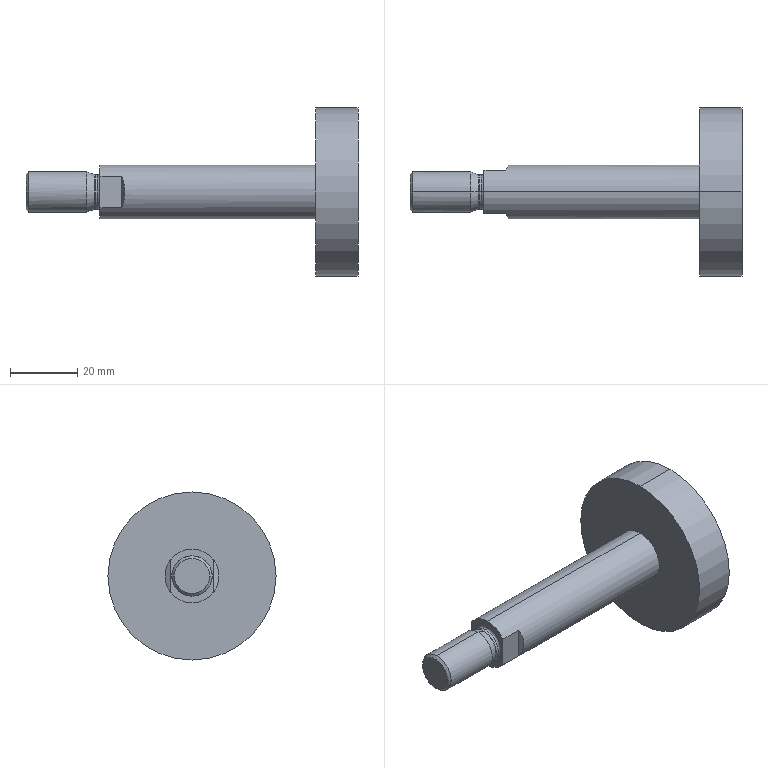Part | SolidWorks | features BaseBody 1 | 1 solid | 24 faces | box 98.8 x 50 x 50 mm | volume 39735 mm3 | cylinder 8 | plane 8 | spline 4 | cone 4 | commonest cylinder face diameters 10.2 x2 12 x2 16 x2 50 x2
STEP:
#1=CARTESIAN_POINT('',(-8.8,0.,5.1));
#2=VERTEX_POINT('',#1);
#3=CARTESIAN_POINT('',(-8.8,0.,-5.1));
#4=VERTEX_POINT('',#3);
#5=CARTESIAN_POINT('',(-8.8,0.,0.));
#6=DIRECTION('',(-1.,0.,0.));
#7=DIRECTION('',(0.,0.,-1.));
#8=AXIS2_PLACEMENT_3D('',#5,#6,#7);
#9=CIRCLE('',#8,5.1);
#10=EDGE_CURVE('',#2,#4,#9,.T.);
#11=ORIENTED_EDGE('',*,*,#10,.F.);
#12=CARTESIAN_POINT('',(-8.2,0.,5.7));
#13=VERTEX_POINT('',#12);
#14=CARTESIAN_POINT('',(-8.8,0.,5.7));
#15=DIRECTION('',(0.,-1.,0.));
#16=DIRECTION('',(0.,0.,1.));
#17=AXIS2_PLACEMENT_3D('',#14,#15,#16);
#18=CIRCLE('',#17,0.6);
#19=EDGE_CURVE('',#2,#13,#18,.T.);
#20=ORIENTED_EDGE('',*,*,#19,.T.);
#21=CARTESIAN_POINT('',(-8.2,0.,-5.7));
#22=VERTEX_POINT('',#21);
#23=CARTESIAN_POINT('',(-8.2,0.,5.7));
#24=CARTESIAN_POINT('',(-8.2,11.4,5.7));
#25=CARTESIAN_POINT('',(-8.2,11.4,-5.7));
#26=CARTESIAN_POINT('',(-8.2,0.,-5.7));
#27=(BOUNDED_CURVE()B_SPLINE_CURVE(3,(#23,#24,#25,#26),.UNSPECIFIED.,.F.,.F.)B_SPLINE_CURVE_WITH_KNOTS((4,4),(0.5,1.),.UNSPECIFIED.)CURVE()GEOMETRIC_REPRESENTATION_ITEM()RATIONAL_B_SPLINE_CURVE((1.,0.3333,0.3333,1.))REPRESENTATION_ITEM(''));
#28=EDGE_CURVE('',#13,#22,#27,.T.);
#29=ORIENTED_EDGE('',*,*,#28,.T.);
#30=CARTESIAN_POINT('',(-8.8,0.,-5.7));
#31=DIRECTION('',(0.,1.,0.));
#32=DIRECTION('',(0.,0.,-1.));
#33=AXIS2_PLACEMENT_3D('',#30,#31,#32);
#34=CIRCLE('',#33,0.6);
#35=EDGE_CURVE('',#4,#22,#34,.T.);
#36=ORIENTED_EDGE('',*,*,#35,.F.);
#37=EDGE_LOOP('',(#11,#20,#29,#36));
#38=FACE_OUTER_BOUND('',#37,.T.);
#39=CARTESIAN_POINT('',(-8.8,0.,-5.1));
#40=CARTESIAN_POINT('',(-8.8,10.2,-5.1));
#41=CARTESIAN_POINT('',(-8.8,10.2,5.1));
#42=CARTESIAN_POINT('',(-8.8,0.,5.1));
#43=CARTESIAN_POINT('',(-8.449,0.,-5.1));
#44=CARTESIAN_POINT('',(-8.449,10.2,-5.1));
#45=CARTESIAN_POINT('',(-8.449,10.2,5.1));
#46=CARTESIAN_POINT('',(-8.449,0.,5.1));
#47=CARTESIAN_POINT('',(-8.2,0.,-5.349));
#48=CARTESIAN_POINT('',(-8.2,10.697,-5.349));
#49=CARTESIAN_POINT('',(-8.2,10.697,5.349));
#50=CARTESIAN_POINT('',(-8.2,0.,5.349));
#51=CARTESIAN_POINT('',(-8.2,0.,-5.7));
#52=CARTESIAN_POINT('',(-8.2,11.4,-5.7));
#53=CARTESIAN_POINT('',(-8.2,11.4,5.7));
#54=CARTESIAN_POINT('',(-8.2,0.,5.7));
#55=(BOUNDED_SURFACE()B_SPLINE_SURFACE(3,3,((#39,#40,#41,#42),(#43,#44,#45,#46),(#47,#48,#49,#50),(#51,#52,#53,#54)),.UNSPECIFIED.,.F.,.F.,.F.)B_SPLINE_SURFACE_WITH_KNOTS((4,4),(4,4),(0.,1.),(0.,1.),.UNSPECIFIED.)GEOMETRIC_REPRESENTATION_ITEM()RATIONAL_B_SPLINE_SURFACE(((1.,0.3333,0.3333,1.),(0.8047,0.2682,0.2682,0.8047),(0.8047,0.2682,0.2682,0.8047),(1.,0.3333,0.3333,1.)))REPRESENTATION_ITEM('')SURFACE());
#56=ADVANCED_FACE('',(#38),#55,.F.);
#57=CARTESIAN_POINT('',(-9.799,0.,5.136));
#58=VERTEX_POINT('',#57);
#59=CARTESIAN_POINT('',(-9.799,0.,-5.136));
#60=VERTEX_POINT('',#59);
#61=CARTESIAN_POINT('',(-9.799,0.,0.));
#62=DIRECTION('',(-1.,0.,0.));
#63=DIRECTION('',(0.,0.,-1.));
#64=AXIS2_PLACEMENT_3D('',#61,#62,#63);
#65=CIRCLE('',#64,5.136);
#66=EDGE_CURVE('',#58,#60,#65,.T.);
#67=ORIENTED_EDGE('',*,*,#66,.F.);
#68=CARTESIAN_POINT('',(-9.594,0.,5.1));
#69=VERTEX_POINT('',#68);
#70=CARTESIAN_POINT('',(-9.594,0.,5.7));
#71=DIRECTION('',(0.,-1.,0.));
#72=DIRECTION('',(0.,0.,1.));
#73=AXIS2_PLACEMENT_3D('',#70,#71,#72);
#74=CIRCLE('',#73,0.6);
#75=EDGE_CURVE('',#58,#69,#74,.T.);
#76=ORIENTED_EDGE('',*,*,#75,.T.);
#77=CARTESIAN_POINT('',(-9.594,0.,-5.1));
#78=VERTEX_POINT('',#77);
#79=CARTESIAN_POINT('',(-9.594,0.,0.));
#80=DIRECTION('',(1.,0.,0.));
#81=DIRECTION('',(0.,0.,1.));
#82=AXIS2_PLACEMENT_3D('',#79,#80,#81);
#83=CIRCLE('',#82,5.1);
#84=EDGE_CURVE('',#78,#69,#83,.T.);
#85=ORIENTED_EDGE('',*,*,#84,.F.);
#86=CARTESIAN_POINT('',(-9.594,0.,-5.7));
#87=DIRECTION('',(0.,1.,0.));
#88=DIRECTION('',(0.,0.,-1.));
#89=AXIS2_PLACEMENT_3D('',#86,#87,#88);
#90=CIRCLE('',#89,0.6);
#91=EDGE_CURVE('',#60,#78,#90,.T.);
#92=ORIENTED_EDGE('',*,*,#91,.F.);
#93=EDGE_LOOP('',(#67,#76,#85,#92));
#94=FACE_OUTER_BOUND('',#93,.T.);
#95=CARTESIAN_POINT('',(-9.799,0.,-5.136));
#96=CARTESIAN_POINT('',(-9.799,10.272,-5.136));
#97=CARTESIAN_POINT('',(-9.799,10.272,5.136));
#98=CARTESIAN_POINT('',(-9.799,0.,5.136));
#99=CARTESIAN_POINT('',(-9.733,0.,-5.112));
#100=CARTESIAN_POINT('',(-9.733,10.224,-5.112));
#101=CARTESIAN_POINT('',(-9.733,10.224,5.112));
#102=CARTESIAN_POINT('',(-9.733,0.,5.112));
#103=CARTESIAN_POINT('',(-9.664,0.,-5.1));
#104=CARTESIAN_POINT('',(-9.664,10.2,-5.1));
#105=CARTESIAN_POINT('',(-9.664,10.2,5.1));
#106=CARTESIAN_POINT('',(-9.664,0.,5.1));
#107=CARTESIAN_POINT('',(-9.594,0.,-5.1));
#108=CARTESIAN_POINT('',(-9.594,10.2,-5.1));
#109=CARTESIAN_POINT('',(-9.594,10.2,5.1));
#110=CARTESIAN_POINT('',(-9.594,0.,5.1));
#111=(BOUNDED_SURFACE()B_SPLINE_SURFACE(3,3,((#95,#96,#97,#98),(#99,#100,#101,#102),(#103,#104,#105,#106),(#107,#108,#109,#110)),.UNSPECIFIED.,.F.,.F.,.T.)B_SPLINE_SURFACE_WITH_KNOTS((4,4),(4,4),(0.,1.),(0.,1.),.UNSPECIFIED.)GEOMETRIC_REPRESENTATION_ITEM()RATIONAL_B_SPLINE_SURFACE(((1.,0.3333,0.3333,1.),(0.9899,0.33,0.33,0.9899),(0.9899,0.33,0.33,0.9899),(1.,0.3333,0.3333,1.)))REPRESENTATION_ITEM('')SURFACE());
#112=ADVANCED_FACE('',(#94),#111,.F.);
#113=CARTESIAN_POINT('',(56.1,0.,8.));
#114=VERTEX_POINT('',#113);
#115=CARTESIAN_POINT('',(56.1,0.,-8.));
#116=VERTEX_POINT('',#115);
#117=CARTESIAN_POINT('',(56.1,0.,0.));
#118=DIRECTION('',(-1.,0.,0.));
#119=DIRECTION('',(0.,0.,1.));
#120=AXIS2_PLACEMENT_3D('',#117,#118,#119);
#121=CIRCLE('',#120,8.);
#122=EDGE_CURVE('',#114,#116,#121,.T.);
#123=ORIENTED_EDGE('',*,*,#122,.T.);
#124=CARTESIAN_POINT('',(-8.2,0.,-8.));
#125=VERTEX_POINT('',#124);
#126=CARTESIAN_POINT('',(68.6,0.,-8.));
#127=DIRECTION('',(-1.,0.,0.));
#128=VECTOR('',#127,1000.);
#129=LINE('',#126,#128);
#130=EDGE_CURVE('',#116,#125,#129,.T.);
#131=ORIENTED_EDGE('',*,*,#130,.T.);
#132=CARTESIAN_POINT('',(-8.2,6.5,-4.664));
#133=VERTEX_POINT('',#132);
#134=CARTESIAN_POINT('',(-8.2,0.,0.));
#135=DIRECTION('',(1.,0.,0.));
#136=DIRECTION('',(0.,0.,1.));
#137=AXIS2_PLACEMENT_3D('',#134,#135,#136);
#138=CIRCLE('',#137,8.);
#139=EDGE_CURVE('',#125,#133,#138,.T.);
#140=ORIENTED_EDGE('',*,*,#139,.T.);
#141=CARTESIAN_POINT('',(-1.7,6.5,-4.664));
#142=VERTEX_POINT('',#141);
#143=CARTESIAN_POINT('',(68.6,6.5,-4.664));
#144=DIRECTION('',(1.,0.,0.));
#145=VECTOR('',#144,1000.);
#146=LINE('',#143,#145);
#147=EDGE_CURVE('',#133,#142,#146,.T.);
#148=ORIENTED_EDGE('',*,*,#147,.T.);
#149=CARTESIAN_POINT('',(-1.7,6.5,4.664));
#150=VERTEX_POINT('',#149);
#151=CARTESIAN_POINT('',(-1.7,6.5,-4.664));
#152=CARTESIAN_POINT('',(-0.5041,8.571,-1.777));
#153=CARTESIAN_POINT('',(-0.5041,8.571,1.777));
#154=CARTESIAN_POINT('',(-1.7,6.5,4.664));
#155=(BOUNDED_CURVE()B_SPLINE_CURVE(3,(#151,#152,#153,#154),.UNSPECIFIED.,.F.,.F.)B_SPLINE_CURVE_WITH_KNOTS((4,4),(2.519,3.764),.UNSPECIFIED.)CURVE()GEOMETRIC_REPRESENTATION_ITEM()RATIONAL_B_SPLINE_CURVE((1.,0.875,0.875,1.))REPRESENTATION_ITEM(''));
#156=EDGE_CURVE('',#142,#150,#155,.T.);
#157=ORIENTED_EDGE('',*,*,#156,.T.);
#158=CARTESIAN_POINT('',(-8.2,6.5,4.664));
#159=VERTEX_POINT('',#158);
#160=CARTESIAN_POINT('',(68.6,6.5,4.664));
#161=DIRECTION('',(-1.,0.,0.));
#162=VECTOR('',#161,1000.);
#163=LINE('',#160,#162);
#164=EDGE_CURVE('',#150,#159,#163,.T.);
#165=ORIENTED_EDGE('',*,*,#164,.T.);
#166=CARTESIAN_POINT('',(-8.2,0.,8.));
#167=VERTEX_POINT('',#166);
#168=CARTESIAN_POINT('',(-8.2,0.,0.));
#169=DIRECTION('',(1.,0.,0.));
#170=DIRECTION('',(0.,0.,1.));
#171=AXIS2_PLACEMENT_3D('',#168,#169,#170);
#172=CIRCLE('',#171,8.);
#173=EDGE_CURVE('',#159,#167,#172,.T.);
#174=ORIENTED_EDGE('',*,*,#173,.T.);
#175=CARTESIAN_POINT('',(68.6,0.,8.));
#176=DIRECTION('',(-1.,0.,0.));
#177=VECTOR('',#176,1000.);
#178=LINE('',#175,#177);
#179=EDGE_CURVE('',#114,#167,#178,.T.);
#180=ORIENTED_EDGE('',*,*,#179,.F.);
#181=EDGE_LOOP('',(#123,#131,#140,#148,#157,#165,#174,#180));
#182=FACE_OUTER_BOUND('',#181,.T.);
#183=CARTESIAN_POINT('',(68.6,0.,0.));
#184=DIRECTION('',(-1.,0.,0.));
#185=DIRECTION('',(0.,0.,1.));
#186=AXIS2_PLACEMENT_3D('',#183,#184,#185);
#187=CYLINDRICAL_SURFACE('',#186,8.);
#188=ADVANCED_FACE('',(#182),#187,.T.);
#189=CARTESIAN_POINT('',(68.6,0.,25.));
#190=VERTEX_POINT('',#189);
#191=CARTESIAN_POINT('',(68.6,0.,-25.));
#192=VERTEX_POINT('',#191);
#193=CARTESIAN_POINT('',(68.6,0.,0.));
#194=DIRECTION('',(-1.,0.,0.));
#195=DIRECTION('',(0.,0.,1.));
#196=AXIS2_PLACEMENT_3D('',#193,#194,#195);
#197=CIRCLE('',#196,25.);
#198=EDGE_CURVE('',#190,#192,#197,.T.);
#199=ORIENTED_EDGE('',*,*,#198,.T.);
#200=CARTESIAN_POINT('',(56.1,0.,-25.));
#201=VERTEX_POINT('',#200);
#202=CARTESIAN_POINT('',(68.6,0.,-25.));
#203=DIRECTION('',(-1.,0.,0.));
#204=VECTOR('',#203,1000.);
#205=LINE('',#202,#204);
#206=EDGE_CURVE('',#192,#201,#205,.T.);
#207=ORIENTED_EDGE('',*,*,#206,.T.);
#208=CARTESIAN_POINT('',(56.1,0.,25.));
#209=VERTEX_POINT('',#208);
#210=CARTESIAN_POINT('',(56.1,0.,0.));
#211=DIRECTION('',(1.,0.,0.));
#212=DIRECTION('',(0.,0.,1.));
#213=AXIS2_PLACEMENT_3D('',#210,#211,#212);
#214=CIRCLE('',#213,25.);
#215=EDGE_CURVE('',#201,#209,#214,.T.);
#216=ORIENTED_EDGE('',*,*,#215,.T.);
#217=CARTESIAN_POINT('',(68.6,0.,25.));
#218=DIRECTION('',(-1.,0.,0.));
#219=VECTOR('',#218,1000.);
#220=LINE('',#217,#219);
#221=EDGE_CURVE('',#190,#209,#220,.T.);
#222=ORIENTED_EDGE('',*,*,#221,.F.);
#223=EDGE_LOOP('',(#199,#207,#216,#222));
#224=FACE_OUTER_BOUND('',#223,.T.);
#225=CARTESIAN_POINT('',(68.6,0.,0.));
#226=DIRECTION('',(-1.,0.,0.));
#227=DIRECTION('',(0.,0.,1.));
#228=AXIS2_PLACEMENT_3D('',#225,#226,#227);
#229=CYLINDRICAL_SURFACE('',#228,25.);
#230=ADVANCED_FACE('',(#224),#229,.T.);
#231=ORIENTED_EDGE('',*,*,#10,.T.);
#232=CARTESIAN_POINT('',(-7.2,0.,-5.1));
#233=DIRECTION('',(-1.,0.,0.));
#234=VECTOR('',#233,1000.);
#235=LINE('',#232,#234);
#236=EDGE_CURVE('',#4,#78,#235,.T.);
#237=ORIENTED_EDGE('',*,*,#236,.T.);
#238=ORIENTED_EDGE('',*,*,#84,.T.);
#239=CARTESIAN_POINT('',(-7.2,0.,5.1));
#240=DIRECTION('',(-1.,0.,0.));
#241=VECTOR('',#240,1000.);
#242=LINE('',#239,#241);
#243=EDGE_CURVE('',#2,#69,#242,.T.);
#244=ORIENTED_EDGE('',*,*,#243,.F.);
#245=EDGE_LOOP('',(#231,#237,#238,#244));
#246=FACE_OUTER_BOUND('',#245,.T.);
#247=CARTESIAN_POINT('',(-7.2,0.,0.));
#248=DIRECTION('',(-1.,0.,0.));
#249=DIRECTION('',(0.,0.,1.));
#250=AXIS2_PLACEMENT_3D('',#247,#248,#249);
#251=CYLINDRICAL_SURFACE('',#250,5.1);
#252=ADVANCED_FACE('',(#246),#251,.T.);
#253=ORIENTED_EDGE('',*,*,#66,.T.);
#254=CARTESIAN_POINT('',(-12.173,0.,-6.));
#255=VERTEX_POINT('',#254);
#256=CARTESIAN_POINT('',(-12.173,0.,-6.));
#257=DIRECTION('',(-0.9397,0.,-0.342));
#258=VECTOR('',#257,1000.);
#259=LINE('',#256,#258);
#260=EDGE_CURVE('',#60,#255,#259,.T.);
#261=ORIENTED_EDGE('',*,*,#260,.T.);
#262=CARTESIAN_POINT('',(-12.173,0.,6.));
#263=VERTEX_POINT('',#262);
#264=CARTESIAN_POINT('',(-12.173,0.,0.));
#265=DIRECTION('',(1.,0.,0.));
#266=DIRECTION('',(0.,0.,1.));
#267=AXIS2_PLACEMENT_3D('',#264,#265,#266);
#268=CIRCLE('',#267,6.);
#269=EDGE_CURVE('',#255,#263,#268,.T.);
#270=ORIENTED_EDGE('',*,*,#269,.T.);
#271=CARTESIAN_POINT('',(-12.173,0.,6.));
#272=DIRECTION('',(-0.9397,0.,0.342));
#273=VECTOR('',#272,1000.);
#274=LINE('',#271,#273);
#275=EDGE_CURVE('',#58,#263,#274,.T.);
#276=ORIENTED_EDGE('',*,*,#275,.F.);
#277=EDGE_LOOP('',(#253,#261,#270,#276));
#278=FACE_OUTER_BOUND('',#277,.T.);
#279=CARTESIAN_POINT('',(-12.173,0.,0.));
#280=DIRECTION('',(-1.,0.,0.));
#281=DIRECTION('',(0.,0.,1.));
#282=AXIS2_PLACEMENT_3D('',#279,#280,#281);
#283=CONICAL_SURFACE('',#282,6.,0.3491);
#284=ADVANCED_FACE('',(#278),#283,.T.);
#285=ORIENTED_EDGE('',*,*,#269,.F.);
#286=CARTESIAN_POINT('',(-29.433,0.,-6.));
#287=VERTEX_POINT('',#286);
#288=CARTESIAN_POINT('',(-7.2,0.,-6.));
#289=DIRECTION('',(-1.,0.,0.));
#290=VECTOR('',#289,1000.);
#291=LINE('',#288,#290);
#292=EDGE_CURVE('',#255,#287,#291,.T.);
#293=ORIENTED_EDGE('',*,*,#292,.T.);
#294=CARTESIAN_POINT('',(-29.433,6.,0.));
#295=VERTEX_POINT('',#294);
#296=CARTESIAN_POINT('',(-29.433,0.,0.));
#297=DIRECTION('',(1.,0.,0.));
#298=DIRECTION('',(0.,0.,1.));
#299=AXIS2_PLACEMENT_3D('',#296,#297,#298);
#300=CIRCLE('',#299,6.);
#301=EDGE_CURVE('',#287,#295,#300,.T.);
#302=ORIENTED_EDGE('',*,*,#301,.T.);
#303=CARTESIAN_POINT('',(-29.433,0.,6.));
#304=VERTEX_POINT('',#303);
#305=CARTESIAN_POINT('',(-29.433,0.,0.));
#306=DIRECTION('',(1.,0.,0.));
#307=DIRECTION('',(0.,0.,1.));
#308=AXIS2_PLACEMENT_3D('',#305,#306,#307);
#309=CIRCLE('',#308,6.);
#310=EDGE_CURVE('',#295,#304,#309,.T.);
#311=ORIENTED_EDGE('',*,*,#310,.T.);
#312=CARTESIAN_POINT('',(-7.2,0.,6.));
#313=DIRECTION('',(-1.,0.,0.));
#314=VECTOR('',#313,1000.);
#315=LINE('',#312,#314);
#316=EDGE_CURVE('',#263,#304,#315,.T.);
#317=ORIENTED_EDGE('',*,*,#316,.F.);
#318=EDGE_LOOP('',(#285,#293,#302,#311,#317));
#319=FACE_OUTER_BOUND('',#318,.T.);
#320=CARTESIAN_POINT('',(-7.2,0.,0.));
#321=DIRECTION('',(-1.,0.,0.));
#322=DIRECTION('',(0.,0.,1.));
#323=AXIS2_PLACEMENT_3D('',#320,#321,#322);
#324=CYLINDRICAL_SURFACE('',#323,6.);
#325=ADVANCED_FACE('',(#319),#324,.T.);
#326=CARTESIAN_POINT('',(-30.2,5.233,0.));
#327=VERTEX_POINT('',#326);
#328=CARTESIAN_POINT('',(-30.2,-5.233,0.));
#329=VERTEX_POINT('',#328);
#330=CARTESIAN_POINT('',(-30.2,0.,0.));
#331=DIRECTION('',(1.,0.,0.));
#332=DIRECTION('',(0.,1.,0.));
#333=AXIS2_PLACEMENT_3D('',#330,#331,#332);
#334=CIRCLE('',#333,5.233);
#335=EDGE_CURVE('',#327,#329,#334,.T.);
#336=ORIENTED_EDGE('',*,*,#335,.T.);
#337=CARTESIAN_POINT('',(-29.433,-6.,0.));
#338=VERTEX_POINT('',#337);
#339=CARTESIAN_POINT('',(-29.433,-6.,0.));
#340=DIRECTION('',(0.7071,-0.7071,0.));
#341=VECTOR('',#340,1000.);
#342=LINE('',#339,#341);
#343=EDGE_CURVE('',#329,#338,#342,.T.);
#344=ORIENTED_EDGE('',*,*,#343,.T.);
#345=CARTESIAN_POINT('',(-29.433,0.,0.));
#346=DIRECTION('',(1.,0.,0.));
#347=DIRECTION('',(0.,0.,1.));
#348=AXIS2_PLACEMENT_3D('',#345,#346,#347);
#349=CIRCLE('',#348,6.);
#350=EDGE_CURVE('',#304,#338,#349,.T.);
#351=ORIENTED_EDGE('',*,*,#350,.F.);
#352=ORIENTED_EDGE('',*,*,#310,.F.);
#353=CARTESIAN_POINT('',(-29.433,6.,0.));
#354=DIRECTION('',(0.7071,0.7071,0.));
#355=VECTOR('',#354,1000.);
#356=LINE('',#353,#355);
#357=EDGE_CURVE('',#327,#295,#356,.T.);
#358=ORIENTED_EDGE('',*,*,#357,.F.);
#359=EDGE_LOOP('',(#336,#344,#351,#352,#358));
#360=FACE_OUTER_BOUND('',#359,.T.);
#361=CARTESIAN_POINT('',(-29.433,0.,0.));
#362=DIRECTION('',(1.,0.,0.));
#363=DIRECTION('',(0.,1.,0.));
#364=AXIS2_PLACEMENT_3D('',#361,#362,#363);
#365=CONICAL_SURFACE('',#364,6.,0.7854);
#366=ADVANCED_FACE('',(#360),#365,.T.);
#367=ORIENTED_EDGE('',*,*,#130,.F.);
#368=CARTESIAN_POINT('',(56.1,0.,0.));
#369=DIRECTION('',(-1.,0.,0.));
#370=DIRECTION('',(0.,0.,1.));
#371=AXIS2_PLACEMENT_3D('',#368,#369,#370);
#372=CIRCLE('',#371,8.);
#373=EDGE_CURVE('',#116,#114,#372,.T.);
#374=ORIENTED_EDGE('',*,*,#373,.T.);
#375=ORIENTED_EDGE('',*,*,#179,.T.);
#376=CARTESIAN_POINT('',(-8.2,-6.5,4.664));
#377=VERTEX_POINT('',#376);
#378=CARTESIAN_POINT('',(-8.2,0.,0.));
#379=DIRECTION('',(1.,0.,0.));
#380=DIRECTION('',(0.,0.,1.));
#381=AXIS2_PLACEMENT_3D('',#378,#379,#380);
#382=CIRCLE('',#381,8.);
#383=EDGE_CURVE('',#167,#377,#382,.T.);
#384=ORIENTED_EDGE('',*,*,#383,.T.);
#385=CARTESIAN_POINT('',(-1.7,-6.5,4.664));
#386=VERTEX_POINT('',#385);
#387=CARTESIAN_POINT('',(68.6,-6.5,4.664));
#388=DIRECTION('',(1.,0.,0.));
#389=VECTOR('',#388,1000.);
#390=LINE('',#387,#389);
#391=EDGE_CURVE('',#377,#386,#390,.T.);
#392=ORIENTED_EDGE('',*,*,#391,.T.);
#393=CARTESIAN_POINT('',(-1.7,-6.5,-4.664));
#394=VERTEX_POINT('',#393);
#395=CARTESIAN_POINT('',(-1.7,-6.5,4.664));
#396=CARTESIAN_POINT('',(-0.5041,-8.571,1.777));
#397=CARTESIAN_POINT('',(-0.5041,-8.571,-1.777));
#398=CARTESIAN_POINT('',(-1.7,-6.5,-4.664));
#399=(BOUNDED_CURVE()B_SPLINE_CURVE(3,(#395,#396,#397,#398),.UNSPECIFIED.,.F.,.F.)B_SPLINE_CURVE_WITH_KNOTS((4,4),(2.519,3.764),.UNSPECIFIED.)CURVE()GEOMETRIC_REPRESENTATION_ITEM()RATIONAL_B_SPLINE_CURVE((1.,0.875,0.875,1.))REPRESENTATION_ITEM(''));
#400=EDGE_CURVE('',#386,#394,#399,.T.);
#401=ORIENTED_EDGE('',*,*,#400,.T.);
#402=CARTESIAN_POINT('',(-8.2,-6.5,-4.664));
#403=VERTEX_POINT('',#402);
#404=CARTESIAN_POINT('',(68.6,-6.5,-4.664));
#405=DIRECTION('',(-1.,0.,0.));
#406=VECTOR('',#405,1000.);
#407=LINE('',#404,#406);
#408=EDGE_CURVE('',#394,#403,#407,.T.);
#409=ORIENTED_EDGE('',*,*,#408,.T.);
#410=CARTESIAN_POINT('',(-8.2,0.,0.));
#411=DIRECTION('',(1.,0.,0.));
#412=DIRECTION('',(0.,0.,1.));
#413=AXIS2_PLACEMENT_3D('',#410,#411,#412);
#414=CIRCLE('',#413,8.);
#415=EDGE_CURVE('',#403,#125,#414,.T.);
#416=ORIENTED_EDGE('',*,*,#415,.T.);
#417=EDGE_LOOP('',(#367,#374,#375,#384,#392,#401,#409,#416));
#418=FACE_OUTER_BOUND('',#417,.T.);
#419=CARTESIAN_POINT('',(68.6,0.,0.));
#420=DIRECTION('',(-1.,0.,0.));
#421=DIRECTION('',(0.,0.,1.));
#422=AXIS2_PLACEMENT_3D('',#419,#420,#421);
#423=CYLINDRICAL_SURFACE('',#422,8.);
#424=ADVANCED_FACE('',(#418),#423,.T.);
#425=ORIENTED_EDGE('',*,*,#400,.F.);
#426=CARTESIAN_POINT('',(-1.7,-6.5,16.));
#427=DIRECTION('',(0.,0.,-1.));
#428=VECTOR('',#427,1000.);
#429=LINE('',#426,#428);
#430=EDGE_CURVE('',#386,#394,#429,.T.);
#431=ORIENTED_EDGE('',*,*,#430,.T.);
#432=EDGE_LOOP('',(#425,#431));
#433=FACE_OUTER_BOUND('',#432,.T.);
#434=CARTESIAN_POINT('',(5.806,-19.5,16.));
#435=DIRECTION('',(-0.866,-0.5,0.));
#436=DIRECTION('',(0.5,-0.866,0.));
#437=AXIS2_PLACEMENT_3D('',#434,#435,#436);
#438=PLANE('',#437);
#439=ADVANCED_FACE('',(#433),#438,.T.);
#440=ORIENTED_EDGE('',*,*,#391,.F.);
#441=CARTESIAN_POINT('',(-8.2,-6.5,16.));
#442=DIRECTION('',(0.,0.,-1.));
#443=VECTOR('',#442,1000.);
#444=LINE('',#441,#443);
#445=EDGE_CURVE('',#377,#403,#444,.T.);
#446=ORIENTED_EDGE('',*,*,#445,.T.);
#447=ORIENTED_EDGE('',*,*,#408,.F.);
#448=ORIENTED_EDGE('',*,*,#430,.F.);
#449=EDGE_LOOP('',(#440,#446,#447,#448));
#450=FACE_OUTER_BOUND('',#449,.T.);
#451=CARTESIAN_POINT('',(-1.7,-6.5,16.));
#452=DIRECTION('',(0.,-1.,0.));
#453=DIRECTION('',(0.,0.,-1.));
#454=AXIS2_PLACEMENT_3D('',#451,#452,#453);
#455=PLANE('',#454);
#456=ADVANCED_FACE('',(#450),#455,.T.);
#457=CARTESIAN_POINT('',(-8.2,0.,-5.7));
#458=CARTESIAN_POINT('',(-8.2,-11.4,-5.7));
#459=CARTESIAN_POINT('',(-8.2,-11.4,5.7));
#460=CARTESIAN_POINT('',(-8.2,0.,5.7));
#461=(BOUNDED_CURVE()B_SPLINE_CURVE(3,(#457,#458,#459,#460),.UNSPECIFIED.,.F.,.T.)B_SPLINE_CURVE_WITH_KNOTS((4,4),(0.,0.5),.UNSPECIFIED.)CURVE()GEOMETRIC_REPRESENTATION_ITEM()RATIONAL_B_SPLINE_CURVE((1.,0.3333,0.3333,1.))REPRESENTATION_ITEM(''));
#462=EDGE_CURVE('',#22,#13,#461,.T.);
#463=ORIENTED_EDGE('',*,*,#462,.F.);
#464=ORIENTED_EDGE('',*,*,#28,.F.);
#465=EDGE_LOOP('',(#463,#464));
#466=FACE_BOUND('',#465,.T.);
#467=CARTESIAN_POINT('',(-8.2,6.5,0.));
#468=DIRECTION('',(0.,0.,1.));
#469=VECTOR('',#468,1000.);
#470=LINE('',#467,#469);
#471=EDGE_CURVE('',#133,#159,#470,.T.);
#472=ORIENTED_EDGE('',*,*,#471,.F.);
#473=ORIENTED_EDGE('',*,*,#139,.F.);
#474=ORIENTED_EDGE('',*,*,#415,.F.);
#475=ORIENTED_EDGE('',*,*,#445,.F.);
#476=ORIENTED_EDGE('',*,*,#383,.F.);
#477=ORIENTED_EDGE('',*,*,#173,.F.);
#478=EDGE_LOOP('',(#472,#473,#474,#475,#476,#477));
#479=FACE_OUTER_BOUND('',#478,.T.);
#480=CARTESIAN_POINT('',(-8.2,0.,0.));
#481=DIRECTION('',(1.,0.,0.));
#482=DIRECTION('',(0.,0.,-1.));
#483=AXIS2_PLACEMENT_3D('',#480,#481,#482);
#484=PLANE('',#483);
#485=ADVANCED_FACE('',(#466,#479),#484,.F.);
#486=ORIENTED_EDGE('',*,*,#147,.F.);
#487=ORIENTED_EDGE('',*,*,#471,.T.);
#488=ORIENTED_EDGE('',*,*,#164,.F.);
#489=CARTESIAN_POINT('',(-1.7,6.5,16.));
#490=DIRECTION('',(0.,0.,-1.));
#491=VECTOR('',#490,1000.);
#492=LINE('',#489,#491);
#493=EDGE_CURVE('',#150,#142,#492,.T.);
#494=ORIENTED_EDGE('',*,*,#493,.T.);
#495=EDGE_LOOP('',(#486,#487,#488,#494));
#496=FACE_OUTER_BOUND('',#495,.T.);
#497=CARTESIAN_POINT('',(-8.2,6.5,16.));
#498=DIRECTION('',(0.,1.,0.));
#499=DIRECTION('',(0.,0.,1.));
#500=AXIS2_PLACEMENT_3D('',#497,#498,#499);
#501=PLANE('',#500);
#502=ADVANCED_FACE('',(#496),#501,.T.);
#503=ORIENTED_EDGE('',*,*,#156,.F.);
#504=ORIENTED_EDGE('',*,*,#493,.F.);
#505=EDGE_LOOP('',(#503,#504));
#506=FACE_OUTER_BOUND('',#505,.T.);
#507=CARTESIAN_POINT('',(-1.7,6.5,16.));
#508=DIRECTION('',(-0.866,0.5,0.));
#509=DIRECTION('',(-0.5,-0.866,0.));
#510=AXIS2_PLACEMENT_3D('',#507,#508,#509);
#511=PLANE('',#510);
#512=ADVANCED_FACE('',(#506),#511,.T.);
#513=ORIENTED_EDGE('',*,*,#122,.F.);
#514=ORIENTED_EDGE('',*,*,#373,.F.);
#515=EDGE_LOOP('',(#513,#514));
#516=FACE_BOUND('',#515,.T.);
#517=CARTESIAN_POINT('',(56.1,0.,0.));
#518=DIRECTION('',(1.,0.,0.));
#519=DIRECTION('',(0.,0.,1.));
#520=AXIS2_PLACEMENT_3D('',#517,#518,#519);
#521=CIRCLE('',#520,25.);
#522=EDGE_CURVE('',#209,#201,#521,.T.);
#523=ORIENTED_EDGE('',*,*,#522,.F.);
#524=ORIENTED_EDGE('',*,*,#215,.F.);
#525=EDGE_LOOP('',(#523,#524));
#526=FACE_OUTER_BOUND('',#525,.T.);
#527=CARTESIAN_POINT('',(56.1,0.,0.));
#528=DIRECTION('',(1.,0.,0.));
#529=DIRECTION('',(0.,0.,-1.));
#530=AXIS2_PLACEMENT_3D('',#527,#528,#529);
#531=PLANE('',#530);
#532=ADVANCED_FACE('',(#516,#526),#531,.F.);
#533=ORIENTED_EDGE('',*,*,#19,.F.);
#534=CARTESIAN_POINT('',(-8.8,0.,0.));
#535=DIRECTION('',(-1.,0.,0.));
#536=DIRECTION('',(0.,0.,-1.));
#537=AXIS2_PLACEMENT_3D('',#534,#535,#536);
#538=CIRCLE('',#537,5.1);
#539=EDGE_CURVE('',#4,#2,#538,.T.);
#540=ORIENTED_EDGE('',*,*,#539,.F.);
#541=ORIENTED_EDGE('',*,*,#35,.T.);
#542=ORIENTED_EDGE('',*,*,#462,.T.);
#543=EDGE_LOOP('',(#533,#540,#541,#542));
#544=FACE_OUTER_BOUND('',#543,.T.);
#545=CARTESIAN_POINT('',(-8.8,0.,5.1));
#546=CARTESIAN_POINT('',(-8.8,-10.2,5.1));
#547=CARTESIAN_POINT('',(-8.8,-10.2,-5.1));
#548=CARTESIAN_POINT('',(-8.8,0.,-5.1));
#549=CARTESIAN_POINT('',(-8.449,0.,5.1));
#550=CARTESIAN_POINT('',(-8.449,-10.2,5.1));
#551=CARTESIAN_POINT('',(-8.449,-10.2,-5.1));
#552=CARTESIAN_POINT('',(-8.449,0.,-5.1));
#553=CARTESIAN_POINT('',(-8.2,0.,5.349));
#554=CARTESIAN_POINT('',(-8.2,-10.697,5.349));
#555=CARTESIAN_POINT('',(-8.2,-10.697,-5.349));
#556=CARTESIAN_POINT('',(-8.2,0.,-5.349));
#557=CARTESIAN_POINT('',(-8.2,0.,5.7));
#558=CARTESIAN_POINT('',(-8.2,-11.4,5.7));
#559=CARTESIAN_POINT('',(-8.2,-11.4,-5.7));
#560=CARTESIAN_POINT('',(-8.2,0.,-5.7));
#561=(BOUNDED_SURFACE()B_SPLINE_SURFACE(3,3,((#545,#546,#547,#548),(#549,#550,#551,#552),(#553,#554,#555,#556),(#557,#558,#559,#560)),.UNSPECIFIED.,.F.,.F.,.F.)B_SPLINE_SURFACE_WITH_KNOTS((4,4),(4,4),(0.,1.),(0.,1.),.UNSPECIFIED.)GEOMETRIC_REPRESENTATION_ITEM()RATIONAL_B_SPLINE_SURFACE(((1.,0.3333,0.3333,1.),(0.8047,0.2682,0.2682,0.8047),(0.8047,0.2682,0.2682,0.8047),(1.,0.3333,0.3333,1.)))REPRESENTATION_ITEM('')SURFACE());
#562=ADVANCED_FACE('',(#544),#561,.F.);
#563=ORIENTED_EDGE('',*,*,#206,.F.);
#564=CARTESIAN_POINT('',(68.6,0.,0.));
#565=DIRECTION('',(-1.,0.,0.));
#566=DIRECTION('',(0.,0.,1.));
#567=AXIS2_PLACEMENT_3D('',#564,#565,#566);
#568=CIRCLE('',#567,25.);
#569=EDGE_CURVE('',#192,#190,#568,.T.);
#570=ORIENTED_EDGE('',*,*,#569,.T.);
#571=ORIENTED_EDGE('',*,*,#221,.T.);
#572=ORIENTED_EDGE('',*,*,#522,.T.);
#573=EDGE_LOOP('',(#563,#570,#571,#572));
#574=FACE_OUTER_BOUND('',#573,.T.);
#575=CARTESIAN_POINT('',(68.6,0.,0.));
#576=DIRECTION('',(-1.,0.,0.));
#577=DIRECTION('',(0.,0.,1.));
#578=AXIS2_PLACEMENT_3D('',#575,#576,#577);
#579=CYLINDRICAL_SURFACE('',#578,25.);
#580=ADVANCED_FACE('',(#574),#579,.T.);
#581=ORIENTED_EDGE('',*,*,#236,.F.);
#582=ORIENTED_EDGE('',*,*,#539,.T.);
#583=ORIENTED_EDGE('',*,*,#243,.T.);
#584=CARTESIAN_POINT('',(-9.594,0.,0.));
#585=DIRECTION('',(1.,0.,0.));
#586=DIRECTION('',(0.,0.,1.));
#587=AXIS2_PLACEMENT_3D('',#584,#585,#586);
#588=CIRCLE('',#587,5.1);
#589=EDGE_CURVE('',#69,#78,#588,.T.);
#590=ORIENTED_EDGE('',*,*,#589,.T.);
#591=EDGE_LOOP('',(#581,#582,#583,#590));
#592=FACE_OUTER_BOUND('',#591,.T.);
#593=CARTESIAN_POINT('',(-7.2,0.,0.));
#594=DIRECTION('',(-1.,0.,0.));
#595=DIRECTION('',(0.,0.,1.));
#596=AXIS2_PLACEMENT_3D('',#593,#594,#595);
#597=CYLINDRICAL_SURFACE('',#596,5.1);
#598=ADVANCED_FACE('',(#592),#597,.T.);
#599=ORIENTED_EDGE('',*,*,#198,.F.);
#600=ORIENTED_EDGE('',*,*,#569,.F.);
#601=EDGE_LOOP('',(#599,#600));
#602=FACE_OUTER_BOUND('',#601,.T.);
#603=CARTESIAN_POINT('',(68.6,8.,0.));
#604=DIRECTION('',(-1.,0.,0.));
#605=DIRECTION('',(0.,0.,1.));
#606=AXIS2_PLACEMENT_3D('',#603,#604,#605);
#607=PLANE('',#606);
#608=ADVANCED_FACE('',(#602),#607,.F.);
#609=ORIENTED_EDGE('',*,*,#75,.F.);
#610=CARTESIAN_POINT('',(-9.799,0.,0.));
#611=DIRECTION('',(-1.,0.,0.));
#612=DIRECTION('',(0.,0.,-1.));
#613=AXIS2_PLACEMENT_3D('',#610,#611,#612);
#614=CIRCLE('',#613,5.136);
#615=EDGE_CURVE('',#60,#58,#614,.T.);
#616=ORIENTED_EDGE('',*,*,#615,.F.);
#617=ORIENTED_EDGE('',*,*,#91,.T.);
#618=ORIENTED_EDGE('',*,*,#589,.F.);
#619=EDGE_LOOP('',(#609,#616,#617,#618));
#620=FACE_OUTER_BOUND('',#619,.T.);
#621=CARTESIAN_POINT('',(-9.799,0.,5.136));
#622=CARTESIAN_POINT('',(-9.799,-10.272,5.136));
#623=CARTESIAN_POINT('',(-9.799,-10.272,-5.136));
#624=CARTESIAN_POINT('',(-9.799,0.,-5.136));
#625=CARTESIAN_POINT('',(-9.733,0.,5.112));
#626=CARTESIAN_POINT('',(-9.733,-10.224,5.112));
#627=CARTESIAN_POINT('',(-9.733,-10.224,-5.112));
#628=CARTESIAN_POINT('',(-9.733,0.,-5.112));
#629=CARTESIAN_POINT('',(-9.664,0.,5.1));
#630=CARTESIAN_POINT('',(-9.664,-10.2,5.1));
#631=CARTESIAN_POINT('',(-9.664,-10.2,-5.1));
#632=CARTESIAN_POINT('',(-9.664,0.,-5.1));
#633=CARTESIAN_POINT('',(-9.594,0.,5.1));
#634=CARTESIAN_POINT('',(-9.594,-10.2,5.1));
#635=CARTESIAN_POINT('',(-9.594,-10.2,-5.1));
#636=CARTESIAN_POINT('',(-9.594,0.,-5.1));
#637=(BOUNDED_SURFACE()B_SPLINE_SURFACE(3,3,((#621,#622,#623,#624),(#625,#626,#627,#628),(#629,#630,#631,#632),(#633,#634,#635,#636)),.UNSPECIFIED.,.F.,.F.,.F.)B_SPLINE_SURFACE_WITH_KNOTS((4,4),(4,4),(0.,1.),(0.,1.),.UNSPECIFIED.)GEOMETRIC_REPRESENTATION_ITEM()RATIONAL_B_SPLINE_SURFACE(((1.,0.3333,0.3333,1.),(0.9899,0.33,0.33,0.9899),(0.9899,0.33,0.33,0.9899),(1.,0.3333,0.3333,1.)))REPRESENTATION_ITEM('')SURFACE());
#638=ADVANCED_FACE('',(#620),#637,.F.);
#639=ORIENTED_EDGE('',*,*,#260,.F.);
#640=ORIENTED_EDGE('',*,*,#615,.T.);
#641=ORIENTED_EDGE('',*,*,#275,.T.);
#642=CARTESIAN_POINT('',(-12.173,0.,0.));
#643=DIRECTION('',(1.,0.,0.));
#644=DIRECTION('',(0.,0.,1.));
#645=AXIS2_PLACEMENT_3D('',#642,#643,#644);
#646=CIRCLE('',#645,6.);
#647=EDGE_CURVE('',#263,#255,#646,.T.);
#648=ORIENTED_EDGE('',*,*,#647,.T.);
#649=EDGE_LOOP('',(#639,#640,#641,#648));
#650=FACE_OUTER_BOUND('',#649,.T.);
#651=CARTESIAN_POINT('',(-12.173,0.,0.));
#652=DIRECTION('',(-1.,0.,0.));
#653=DIRECTION('',(0.,0.,1.));
#654=AXIS2_PLACEMENT_3D('',#651,#652,#653);
#655=CONICAL_SURFACE('',#654,6.,0.3491);
#656=ADVANCED_FACE('',(#650),#655,.T.);
#657=ORIENTED_EDGE('',*,*,#292,.F.);
#658=ORIENTED_EDGE('',*,*,#647,.F.);
#659=ORIENTED_EDGE('',*,*,#316,.T.);
#660=ORIENTED_EDGE('',*,*,#350,.T.);
#661=CARTESIAN_POINT('',(-29.433,0.,0.));
#662=DIRECTION('',(1.,0.,0.));
#663=DIRECTION('',(0.,0.,1.));
#664=AXIS2_PLACEMENT_3D('',#661,#662,#663);
#665=CIRCLE('',#664,6.);
#666=EDGE_CURVE('',#338,#287,#665,.T.);
#667=ORIENTED_EDGE('',*,*,#666,.T.);
#668=EDGE_LOOP('',(#657,#658,#659,#660,#667));
#669=FACE_OUTER_BOUND('',#668,.T.);
#670=CARTESIAN_POINT('',(-7.2,0.,0.));
#671=DIRECTION('',(-1.,0.,0.));
#672=DIRECTION('',(0.,0.,1.));
#673=AXIS2_PLACEMENT_3D('',#670,#671,#672);
#674=CYLINDRICAL_SURFACE('',#673,6.);
#675=ADVANCED_FACE('',(#669),#674,.T.);
#676=ORIENTED_EDGE('',*,*,#343,.F.);
#677=CARTESIAN_POINT('',(-30.2,0.,0.));
#678=DIRECTION('',(1.,0.,0.));
#679=DIRECTION('',(0.,1.,0.));
#680=AXIS2_PLACEMENT_3D('',#677,#678,#679);
#681=CIRCLE('',#680,5.233);
#682=EDGE_CURVE('',#329,#327,#681,.T.);
#683=ORIENTED_EDGE('',*,*,#682,.T.);
#684=ORIENTED_EDGE('',*,*,#357,.T.);
#685=ORIENTED_EDGE('',*,*,#301,.F.);
#686=ORIENTED_EDGE('',*,*,#666,.F.);
#687=EDGE_LOOP('',(#676,#683,#684,#685,#686));
#688=FACE_OUTER_BOUND('',#687,.T.);
#689=CARTESIAN_POINT('',(-29.433,0.,0.));
#690=DIRECTION('',(1.,0.,0.));
#691=DIRECTION('',(0.,1.,0.));
#692=AXIS2_PLACEMENT_3D('',#689,#690,#691);
#693=CONICAL_SURFACE('',#692,6.,0.7854);
#694=ADVANCED_FACE('',(#688),#693,.T.);
#695=ORIENTED_EDGE('',*,*,#335,.F.);
#696=ORIENTED_EDGE('',*,*,#682,.F.);
#697=EDGE_LOOP('',(#695,#696));
#698=FACE_OUTER_BOUND('',#697,.T.);
#699=CARTESIAN_POINT('',(-30.2,0.,0.));
#700=DIRECTION('',(1.,0.,0.));
#701=DIRECTION('',(0.,0.,-1.));
#702=AXIS2_PLACEMENT_3D('',#699,#700,#701);
#703=PLANE('',#702);
#704=ADVANCED_FACE('',(#698),#703,.F.);
#705=CLOSED_SHELL('',(#56,#112,#188,#230,#252,#284,#325,#366,#424,#439,#456,#485,#502,#512,#532,#562,#580,#598,#608,#638,#656,#675,#694,#704));
#706=MANIFOLD_SOLID_BREP('',#705);
#707=CARTESIAN_POINT('',(0.,0.,0.));
#708=DIRECTION('',(0.,0.,1.));
#709=DIRECTION('',(1.,0.,0.));
#710=AXIS2_PLACEMENT_3D('',#707,#708,#709);
#711=(LENGTH_UNIT()NAMED_UNIT(*)SI_UNIT(.MILLI.,.METRE.));
#712=UNCERTAINTY_MEASURE_WITH_UNIT(LENGTH_MEASURE(0.00001),#711,'','');
#713=(NAMED_UNIT(*)PLANE_ANGLE_UNIT()SI_UNIT($,.RADIAN.));
#714=(NAMED_UNIT(*)SI_UNIT($,.STERADIAN.)SOLID_ANGLE_UNIT());
#715=(GEOMETRIC_REPRESENTATION_CONTEXT(3)GLOBAL_UNCERTAINTY_ASSIGNED_CONTEXT((#712))GLOBAL_UNIT_ASSIGNED_CONTEXT((#711,#713,#714))REPRESENTATION_CONTEXT('',''));
#716=ADVANCED_BREP_SHAPE_REPRESENTATION('',(#706,#710),#715);